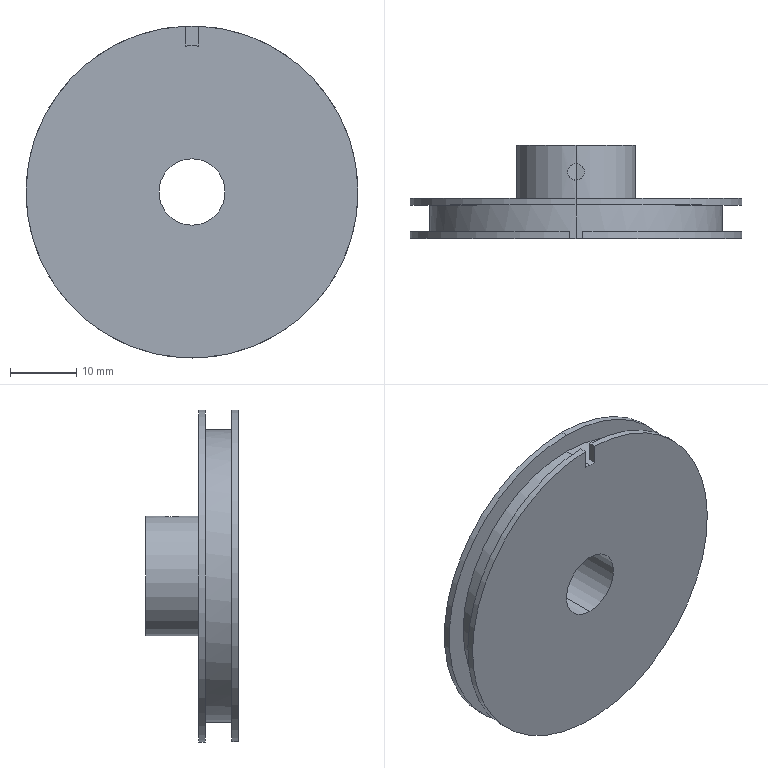Part | SolidWorks | features 3DProfileFeature 1, HoleWzd 1, ICE 1, Revolution 1 | 1 solid | 18 faces | box 50 x 14 x 50 mm | volume 10920 mm3 | cylinder 11 | plane 7 | commonest cylinder face diameters 50 x3 2.5 x2 10 x2 18 x2 44 x2
STEP:
#1=CARTESIAN_POINT('',(0.,-5.25,5.));
#2=VERTEX_POINT('',#1);
#3=CARTESIAN_POINT('',(-1.25,-4.,4.841));
#4=VERTEX_POINT('',#3);
#5=CARTESIAN_POINT('',(0.,-5.25,5.));
#6=CARTESIAN_POINT('',(-0.1659,-5.25,5.));
#7=CARTESIAN_POINT('',(-0.3287,-5.217,4.991));
#8=CARTESIAN_POINT('',(-0.6313,-5.091,4.962));
#9=CARTESIAN_POINT('',(-0.7695,-4.998,4.942));
#10=CARTESIAN_POINT('',(-0.9991,-4.769,4.901));
#11=CARTESIAN_POINT('',(-1.092,-4.63,4.88));
#12=CARTESIAN_POINT('',(-1.217,-4.329,4.85));
#13=CARTESIAN_POINT('',(-1.25,-4.164,4.841));
#14=CARTESIAN_POINT('',(-1.25,-4.,4.841));
#15=B_SPLINE_CURVE_WITH_KNOTS('',3,(#5,#6,#7,#8,#9,#10,#11,#12,#13,#14),.UNSPECIFIED.,.F.,.F.,(4,2,2,2,4),(0.,0.0004906,0.0009812,0.001472,0.001962),.UNSPECIFIED.);
#16=EDGE_CURVE('',#2,#4,#15,.T.);
#17=ORIENTED_EDGE('',*,*,#16,.T.);
#18=CARTESIAN_POINT('',(-1.25,-4.,8.913));
#19=VERTEX_POINT('',#18);
#20=CARTESIAN_POINT('',(-1.25,-4.,9.));
#21=DIRECTION('',(0.,0.,1.));
#22=VECTOR('',#21,1000.);
#23=LINE('',#20,#22);
#24=EDGE_CURVE('',#4,#19,#23,.T.);
#25=ORIENTED_EDGE('',*,*,#24,.T.);
#26=CARTESIAN_POINT('',(0.,-5.25,9.));
#27=VERTEX_POINT('',#26);
#28=CARTESIAN_POINT('',(-1.25,-4.,8.913));
#29=CARTESIAN_POINT('',(-1.25,-4.165,8.913));
#30=CARTESIAN_POINT('',(-1.217,-4.328,8.918));
#31=CARTESIAN_POINT('',(-1.092,-4.63,8.934));
#32=CARTESIAN_POINT('',(-0.9992,-4.768,8.945));
#33=CARTESIAN_POINT('',(-0.7692,-4.999,8.968));
#34=CARTESIAN_POINT('',(-0.63,-5.092,8.979));
#35=CARTESIAN_POINT('',(-0.3295,-5.217,8.995));
#36=CARTESIAN_POINT('',(-0.1653,-5.25,9.));
#37=CARTESIAN_POINT('',(0.,-5.25,9.));
#38=B_SPLINE_CURVE_WITH_KNOTS('',3,(#28,#29,#30,#31,#32,#33,#34,#35,#36,#37),.UNSPECIFIED.,.F.,.F.,(4,2,2,2,4),(0.00587,0.006358,0.006847,0.007336,0.007825),.UNSPECIFIED.);
#39=EDGE_CURVE('',#19,#27,#38,.T.);
#40=ORIENTED_EDGE('',*,*,#39,.T.);
#41=CARTESIAN_POINT('',(1.25,-4.,8.913));
#42=VERTEX_POINT('',#41);
#43=CARTESIAN_POINT('',(0.,-5.25,9.));
#44=CARTESIAN_POINT('',(0.1654,-5.25,9.));
#45=CARTESIAN_POINT('',(0.3278,-5.217,8.995));
#46=CARTESIAN_POINT('',(0.6305,-5.092,8.979));
#47=CARTESIAN_POINT('',(0.7691,-4.999,8.968));
#48=CARTESIAN_POINT('',(0.9994,-4.768,8.945));
#49=CARTESIAN_POINT('',(1.092,-4.629,8.934));
#50=CARTESIAN_POINT('',(1.217,-4.328,8.918));
#51=CARTESIAN_POINT('',(1.25,-4.163,8.913));
#52=CARTESIAN_POINT('',(1.25,-4.,8.913));
#53=B_SPLINE_CURVE_WITH_KNOTS('',3,(#43,#44,#45,#46,#47,#48,#49,#50,#51,#52),.UNSPECIFIED.,.F.,.F.,(4,2,2,2,4),(0.,0.0004892,0.0009784,0.001468,0.001957),.UNSPECIFIED.);
#54=EDGE_CURVE('',#27,#42,#53,.T.);
#55=ORIENTED_EDGE('',*,*,#54,.T.);
#56=CARTESIAN_POINT('',(1.25,-4.,4.841));
#57=VERTEX_POINT('',#56);
#58=CARTESIAN_POINT('',(1.25,-4.,9.));
#59=DIRECTION('',(0.,0.,1.));
#60=VECTOR('',#59,1000.);
#61=LINE('',#58,#60);
#62=EDGE_CURVE('',#57,#42,#61,.T.);
#63=ORIENTED_EDGE('',*,*,#62,.F.);
#64=CARTESIAN_POINT('',(1.25,-4.,4.841));
#65=CARTESIAN_POINT('',(1.25,-4.082,4.841));
#66=CARTESIAN_POINT('',(1.242,-4.164,4.843));
#67=CARTESIAN_POINT('',(1.21,-4.324,4.851));
#68=CARTESIAN_POINT('',(1.186,-4.404,4.857));
#69=CARTESIAN_POINT('',(1.092,-4.63,4.88));
#70=CARTESIAN_POINT('',(0.9989,-4.769,4.901));
#71=CARTESIAN_POINT('',(0.7696,-4.998,4.942));
#72=CARTESIAN_POINT('',(0.6309,-5.091,4.962));
#73=CARTESIAN_POINT('',(0.3301,-5.217,4.991));
#74=CARTESIAN_POINT('',(0.1658,-5.25,5.));
#75=CARTESIAN_POINT('',(0.,-5.25,5.));
#76=B_SPLINE_CURVE_WITH_KNOTS('',3,(#64,#65,#66,#67,#68,#69,#70,#71,#72,#73,#74,#75),.UNSPECIFIED.,.F.,.F.,(4,2,2,2,2,4),(0.005885,0.006131,0.006376,0.006866,0.007356,0.007846),.UNSPECIFIED.);
#77=EDGE_CURVE('',#57,#2,#76,.T.);
#78=ORIENTED_EDGE('',*,*,#77,.T.);
#79=EDGE_LOOP('',(#17,#25,#40,#55,#63,#78));
#80=FACE_OUTER_BOUND('',#79,.T.);
#81=CARTESIAN_POINT('',(0.,-4.,9.));
#82=DIRECTION('',(0.,0.,1.));
#83=DIRECTION('',(1.,0.,0.));
#84=AXIS2_PLACEMENT_3D('',#81,#82,#83);
#85=CYLINDRICAL_SURFACE('',#84,1.25);
#86=ADVANCED_FACE('',(#80),#85,.F.);
#87=CARTESIAN_POINT('',(1.,-13.,21.977));
#88=VERTEX_POINT('',#87);
#89=CARTESIAN_POINT('',(0.,-13.,-22.));
#90=VERTEX_POINT('',#89);
#91=CARTESIAN_POINT('',(0.,-13.,0.));
#92=DIRECTION('',(0.,1.,0.));
#93=DIRECTION('',(0.,0.,1.));
#94=AXIS2_PLACEMENT_3D('',#91,#92,#93);
#95=CIRCLE('',#94,22.);
#96=EDGE_CURVE('',#88,#90,#95,.T.);
#97=ORIENTED_EDGE('',*,*,#96,.T.);
#98=CARTESIAN_POINT('',(0.,-9.,-22.));
#99=VERTEX_POINT('',#98);
#100=CARTESIAN_POINT('',(0.,0.,-22.));
#101=DIRECTION('',(0.,1.,0.));
#102=VECTOR('',#101,1000.);
#103=LINE('',#100,#102);
#104=EDGE_CURVE('',#90,#99,#103,.T.);
#105=ORIENTED_EDGE('',*,*,#104,.T.);
#106=CARTESIAN_POINT('',(0.,-9.,22.));
#107=VERTEX_POINT('',#106);
#108=CARTESIAN_POINT('',(0.,-9.,0.));
#109=DIRECTION('',(0.,1.,0.));
#110=DIRECTION('',(0.,0.,1.));
#111=AXIS2_PLACEMENT_3D('',#108,#109,#110);
#112=CIRCLE('',#111,22.);
#113=EDGE_CURVE('',#107,#99,#112,.T.);
#114=ORIENTED_EDGE('',*,*,#113,.F.);
#115=CARTESIAN_POINT('',(0.,-14.,22.));
#116=VERTEX_POINT('',#115);
#117=CARTESIAN_POINT('',(0.,0.,22.));
#118=DIRECTION('',(0.,1.,0.));
#119=VECTOR('',#118,1000.);
#120=LINE('',#117,#119);
#121=EDGE_CURVE('',#116,#107,#120,.T.);
#122=ORIENTED_EDGE('',*,*,#121,.F.);
#123=CARTESIAN_POINT('',(1.,-14.,21.977));
#124=VERTEX_POINT('',#123);
#125=CARTESIAN_POINT('',(0.,-14.,0.));
#126=DIRECTION('',(0.,1.,0.));
#127=DIRECTION('',(0.,0.,-1.));
#128=AXIS2_PLACEMENT_3D('',#125,#126,#127);
#129=CIRCLE('',#128,22.);
#130=EDGE_CURVE('',#116,#124,#129,.T.);
#131=ORIENTED_EDGE('',*,*,#130,.T.);
#132=CARTESIAN_POINT('',(1.,-23.,21.977));
#133=DIRECTION('',(0.,1.,0.));
#134=VECTOR('',#133,1000.);
#135=LINE('',#132,#134);
#136=EDGE_CURVE('',#124,#88,#135,.T.);
#137=ORIENTED_EDGE('',*,*,#136,.T.);
#138=EDGE_LOOP('',(#97,#105,#114,#122,#131,#137));
#139=FACE_OUTER_BOUND('',#138,.T.);
#140=CARTESIAN_POINT('',(0.,0.,0.));
#141=DIRECTION('',(0.,1.,0.));
#142=DIRECTION('',(0.,0.,1.));
#143=AXIS2_PLACEMENT_3D('',#140,#141,#142);
#144=CYLINDRICAL_SURFACE('',#143,22.);
#145=ADVANCED_FACE('',(#139),#144,.T.);
#146=CARTESIAN_POINT('',(0.,-9.,25.));
#147=VERTEX_POINT('',#146);
#148=CARTESIAN_POINT('',(0.,-9.,-25.));
#149=VERTEX_POINT('',#148);
#150=CARTESIAN_POINT('',(0.,-9.,0.));
#151=DIRECTION('',(0.,1.,0.));
#152=DIRECTION('',(0.,0.,1.));
#153=AXIS2_PLACEMENT_3D('',#150,#151,#152);
#154=CIRCLE('',#153,25.);
#155=EDGE_CURVE('',#147,#149,#154,.T.);
#156=ORIENTED_EDGE('',*,*,#155,.T.);
#157=CARTESIAN_POINT('',(0.,-8.,-25.));
#158=VERTEX_POINT('',#157);
#159=CARTESIAN_POINT('',(0.,0.,-25.));
#160=DIRECTION('',(0.,1.,0.));
#161=VECTOR('',#160,1000.);
#162=LINE('',#159,#161);
#163=EDGE_CURVE('',#149,#158,#162,.T.);
#164=ORIENTED_EDGE('',*,*,#163,.T.);
#165=CARTESIAN_POINT('',(0.,-8.,25.));
#166=VERTEX_POINT('',#165);
#167=CARTESIAN_POINT('',(0.,-8.,0.));
#168=DIRECTION('',(0.,1.,0.));
#169=DIRECTION('',(0.,0.,1.));
#170=AXIS2_PLACEMENT_3D('',#167,#168,#169);
#171=CIRCLE('',#170,25.);
#172=EDGE_CURVE('',#166,#158,#171,.T.);
#173=ORIENTED_EDGE('',*,*,#172,.F.);
#174=CARTESIAN_POINT('',(0.,0.,25.));
#175=DIRECTION('',(0.,1.,0.));
#176=VECTOR('',#175,1000.);
#177=LINE('',#174,#176);
#178=EDGE_CURVE('',#147,#166,#177,.T.);
#179=ORIENTED_EDGE('',*,*,#178,.F.);
#180=EDGE_LOOP('',(#156,#164,#173,#179));
#181=FACE_OUTER_BOUND('',#180,.T.);
#182=CARTESIAN_POINT('',(0.,0.,0.));
#183=DIRECTION('',(0.,1.,0.));
#184=DIRECTION('',(0.,0.,1.));
#185=AXIS2_PLACEMENT_3D('',#182,#183,#184);
#186=CYLINDRICAL_SURFACE('',#185,25.);
#187=ADVANCED_FACE('',(#181),#186,.T.);
#188=CARTESIAN_POINT('',(0.,-8.,9.));
#189=VERTEX_POINT('',#188);
#190=CARTESIAN_POINT('',(0.,-8.,-9.));
#191=VERTEX_POINT('',#190);
#192=CARTESIAN_POINT('',(0.,-8.,0.));
#193=DIRECTION('',(0.,1.,0.));
#194=DIRECTION('',(0.,0.,1.));
#195=AXIS2_PLACEMENT_3D('',#192,#193,#194);
#196=CIRCLE('',#195,9.);
#197=EDGE_CURVE('',#189,#191,#196,.T.);
#198=ORIENTED_EDGE('',*,*,#197,.T.);
#199=CARTESIAN_POINT('',(0.,0.,-9.));
#200=VERTEX_POINT('',#199);
#201=CARTESIAN_POINT('',(0.,0.,-9.));
#202=DIRECTION('',(0.,1.,0.));
#203=VECTOR('',#202,1000.);
#204=LINE('',#201,#203);
#205=EDGE_CURVE('',#191,#200,#204,.T.);
#206=ORIENTED_EDGE('',*,*,#205,.T.);
#207=CARTESIAN_POINT('',(0.,0.,9.));
#208=VERTEX_POINT('',#207);
#209=CARTESIAN_POINT('',(0.,0.,0.));
#210=DIRECTION('',(0.,1.,0.));
#211=DIRECTION('',(0.,0.,1.));
#212=AXIS2_PLACEMENT_3D('',#209,#210,#211);
#213=CIRCLE('',#212,9.);
#214=EDGE_CURVE('',#208,#200,#213,.T.);
#215=ORIENTED_EDGE('',*,*,#214,.F.);
#216=CARTESIAN_POINT('',(0.,-2.75,9.));
#217=VERTEX_POINT('',#216);
#218=CARTESIAN_POINT('',(0.,0.,9.));
#219=DIRECTION('',(0.,1.,0.));
#220=VECTOR('',#219,1000.);
#221=LINE('',#218,#220);
#222=EDGE_CURVE('',#217,#208,#221,.T.);
#223=ORIENTED_EDGE('',*,*,#222,.F.);
#224=CARTESIAN_POINT('',(1.25,-4.,8.913));
#225=CARTESIAN_POINT('',(1.25,-3.918,8.913));
#226=CARTESIAN_POINT('',(1.242,-3.835,8.914));
#227=CARTESIAN_POINT('',(1.21,-3.675,8.918));
#228=CARTESIAN_POINT('',(1.186,-3.597,8.922));
#229=CARTESIAN_POINT('',(1.092,-3.37,8.934));
#230=CARTESIAN_POINT('',(1.,-3.233,8.945));
#231=CARTESIAN_POINT('',(0.7672,-3.,8.968));
#232=CARTESIAN_POINT('',(0.6297,-2.908,8.979));
#233=CARTESIAN_POINT('',(0.4028,-2.814,8.991));
#234=CARTESIAN_POINT('',(0.3249,-2.79,8.994));
#235=CARTESIAN_POINT('',(0.1645,-2.758,8.999));
#236=CARTESIAN_POINT('',(0.08161,-2.75,9.));
#237=CARTESIAN_POINT('',(0.,-2.75,9.));
#238=B_SPLINE_CURVE_WITH_KNOTS('',3,(#224,#225,#226,#227,#228,#229,#230,#231,#232,#233,#234,#235,#236,#237),.UNSPECIFIED.,.F.,.F.,(4,2,2,2,2,2,4),(0.001957,0.002201,0.002446,0.002935,0.003424,0.003668,0.003913),.UNSPECIFIED.);
#239=EDGE_CURVE('',#42,#217,#238,.T.);
#240=ORIENTED_EDGE('',*,*,#239,.F.);
#241=ORIENTED_EDGE('',*,*,#54,.F.);
#242=CARTESIAN_POINT('',(0.,0.,9.));
#243=DIRECTION('',(0.,1.,0.));
#244=VECTOR('',#243,1000.);
#245=LINE('',#242,#244);
#246=EDGE_CURVE('',#189,#27,#245,.T.);
#247=ORIENTED_EDGE('',*,*,#246,.F.);
#248=EDGE_LOOP('',(#198,#206,#215,#223,#240,#241,#247));
#249=FACE_OUTER_BOUND('',#248,.T.);
#250=CARTESIAN_POINT('',(0.,0.,0.));
#251=DIRECTION('',(0.,1.,0.));
#252=DIRECTION('',(0.,0.,1.));
#253=AXIS2_PLACEMENT_3D('',#250,#251,#252);
#254=CYLINDRICAL_SURFACE('',#253,9.);
#255=ADVANCED_FACE('',(#249),#254,.T.);
#256=CARTESIAN_POINT('',(0.,-14.,-5.));
#257=VERTEX_POINT('',#256);
#258=CARTESIAN_POINT('',(0.,-14.,5.));
#259=VERTEX_POINT('',#258);
#260=CARTESIAN_POINT('',(0.,-14.,0.));
#261=DIRECTION('',(0.,1.,0.));
#262=DIRECTION('',(0.,0.,1.));
#263=AXIS2_PLACEMENT_3D('',#260,#261,#262);
#264=CIRCLE('',#263,5.);
#265=EDGE_CURVE('',#257,#259,#264,.T.);
#266=ORIENTED_EDGE('',*,*,#265,.F.);
#267=CARTESIAN_POINT('',(0.,0.,-5.));
#268=VERTEX_POINT('',#267);
#269=CARTESIAN_POINT('',(0.,0.,-5.));
#270=DIRECTION('',(0.,1.,0.));
#271=VECTOR('',#270,1000.);
#272=LINE('',#269,#271);
#273=EDGE_CURVE('',#257,#268,#272,.T.);
#274=ORIENTED_EDGE('',*,*,#273,.T.);
#275=CARTESIAN_POINT('',(0.,0.,5.));
#276=VERTEX_POINT('',#275);
#277=CARTESIAN_POINT('',(0.,0.,0.));
#278=DIRECTION('',(0.,1.,0.));
#279=DIRECTION('',(0.,0.,1.));
#280=AXIS2_PLACEMENT_3D('',#277,#278,#279);
#281=CIRCLE('',#280,5.);
#282=EDGE_CURVE('',#268,#276,#281,.T.);
#283=ORIENTED_EDGE('',*,*,#282,.T.);
#284=CARTESIAN_POINT('',(0.,-2.75,5.));
#285=VERTEX_POINT('',#284);
#286=CARTESIAN_POINT('',(0.,0.,5.));
#287=DIRECTION('',(0.,1.,0.));
#288=VECTOR('',#287,1000.);
#289=LINE('',#286,#288);
#290=EDGE_CURVE('',#285,#276,#289,.T.);
#291=ORIENTED_EDGE('',*,*,#290,.F.);
#292=CARTESIAN_POINT('',(-1.25,-4.,4.841));
#293=CARTESIAN_POINT('',(-1.25,-3.918,4.841));
#294=CARTESIAN_POINT('',(-1.242,-3.835,4.843));
#295=CARTESIAN_POINT('',(-1.21,-3.674,4.852));
#296=CARTESIAN_POINT('',(-1.186,-3.596,4.857));
#297=CARTESIAN_POINT('',(-1.091,-3.369,4.88));
#298=CARTESIAN_POINT('',(-0.9993,-3.231,4.901));
#299=CARTESIAN_POINT('',(-0.8256,-3.058,4.932));
#300=CARTESIAN_POINT('',(-0.7628,-3.006,4.942));
#301=CARTESIAN_POINT('',(-0.6277,-2.916,4.961));
#302=CARTESIAN_POINT('',(-0.5545,-2.877,4.97));
#303=CARTESIAN_POINT('',(-0.3282,-2.783,4.992));
#304=CARTESIAN_POINT('',(-0.1635,-2.75,5.));
#305=CARTESIAN_POINT('',(0.,-2.75,5.));
#306=B_SPLINE_CURVE_WITH_KNOTS('',3,(#292,#293,#294,#295,#296,#297,#298,#299,#300,#301,#302,#303,#304,#305),.UNSPECIFIED.,.F.,.F.,(4,2,2,2,2,2,4),(0.001962,0.002208,0.002453,0.002943,0.003188,0.003433,0.003924),.UNSPECIFIED.);
#307=EDGE_CURVE('',#4,#285,#306,.T.);
#308=ORIENTED_EDGE('',*,*,#307,.F.);
#309=ORIENTED_EDGE('',*,*,#16,.F.);
#310=CARTESIAN_POINT('',(0.,0.,5.));
#311=DIRECTION('',(0.,1.,0.));
#312=VECTOR('',#311,1000.);
#313=LINE('',#310,#312);
#314=EDGE_CURVE('',#259,#2,#313,.T.);
#315=ORIENTED_EDGE('',*,*,#314,.F.);
#316=EDGE_LOOP('',(#266,#274,#283,#291,#308,#309,#315));
#317=FACE_OUTER_BOUND('',#316,.T.);
#318=CARTESIAN_POINT('',(0.,0.,0.));
#319=DIRECTION('',(0.,1.,0.));
#320=DIRECTION('',(0.,0.,1.));
#321=AXIS2_PLACEMENT_3D('',#318,#319,#320);
#322=CYLINDRICAL_SURFACE('',#321,5.);
#323=ADVANCED_FACE('',(#317),#322,.F.);
#324=CARTESIAN_POINT('',(0.,-14.,0.));
#325=DIRECTION('',(0.,1.,0.));
#326=DIRECTION('',(0.,0.,1.));
#327=AXIS2_PLACEMENT_3D('',#324,#325,#326);
#328=CIRCLE('',#327,5.);
#329=EDGE_CURVE('',#259,#257,#328,.T.);
#330=ORIENTED_EDGE('',*,*,#329,.T.);
#331=ORIENTED_EDGE('',*,*,#265,.T.);
#332=EDGE_LOOP('',(#330,#331));
#333=FACE_BOUND('',#332,.T.);
#334=CARTESIAN_POINT('',(1.,-14.,24.98));
#335=VERTEX_POINT('',#334);
#336=CARTESIAN_POINT('',(1.,-14.,0.));
#337=DIRECTION('',(0.,0.,1.));
#338=VECTOR('',#337,1000.);
#339=LINE('',#336,#338);
#340=EDGE_CURVE('',#124,#335,#339,.T.);
#341=ORIENTED_EDGE('',*,*,#340,.F.);
#342=ORIENTED_EDGE('',*,*,#130,.F.);
#343=CARTESIAN_POINT('',(-1.,-14.,21.977));
#344=VERTEX_POINT('',#343);
#345=CARTESIAN_POINT('',(0.,-14.,0.));
#346=DIRECTION('',(0.,1.,0.));
#347=DIRECTION('',(0.,0.,-1.));
#348=AXIS2_PLACEMENT_3D('',#345,#346,#347);
#349=CIRCLE('',#348,22.);
#350=EDGE_CURVE('',#344,#116,#349,.T.);
#351=ORIENTED_EDGE('',*,*,#350,.F.);
#352=CARTESIAN_POINT('',(-1.,-14.,24.98));
#353=VERTEX_POINT('',#352);
#354=CARTESIAN_POINT('',(-1.,-14.,0.));
#355=DIRECTION('',(0.,0.,-1.));
#356=VECTOR('',#355,1000.);
#357=LINE('',#354,#356);
#358=EDGE_CURVE('',#353,#344,#357,.T.);
#359=ORIENTED_EDGE('',*,*,#358,.F.);
#360=CARTESIAN_POINT('',(0.,-14.,0.));
#361=DIRECTION('',(0.,1.,0.));
#362=DIRECTION('',(0.,0.,1.));
#363=AXIS2_PLACEMENT_3D('',#360,#361,#362);
#364=CIRCLE('',#363,25.);
#365=EDGE_CURVE('',#335,#353,#364,.T.);
#366=ORIENTED_EDGE('',*,*,#365,.F.);
#367=EDGE_LOOP('',(#341,#342,#351,#359,#366));
#368=FACE_OUTER_BOUND('',#367,.T.);
#369=CARTESIAN_POINT('',(-25.,-14.,0.));
#370=DIRECTION('',(0.,-1.,0.));
#371=DIRECTION('',(0.,0.,-1.));
#372=AXIS2_PLACEMENT_3D('',#369,#370,#371);
#373=PLANE('',#372);
#374=ADVANCED_FACE('',(#333,#368),#373,.T.);
#375=ORIENTED_EDGE('',*,*,#273,.F.);
#376=ORIENTED_EDGE('',*,*,#329,.F.);
#377=ORIENTED_EDGE('',*,*,#314,.T.);
#378=ORIENTED_EDGE('',*,*,#77,.F.);
#379=CARTESIAN_POINT('',(0.,-2.75,5.));
#380=CARTESIAN_POINT('',(0.1635,-2.75,5.));
#381=CARTESIAN_POINT('',(0.3287,-2.783,4.991));
#382=CARTESIAN_POINT('',(0.6298,-2.908,4.962));
#383=CARTESIAN_POINT('',(0.7684,-3.001,4.942));
#384=CARTESIAN_POINT('',(0.999,-3.231,4.901));
#385=CARTESIAN_POINT('',(1.091,-3.368,4.88));
#386=CARTESIAN_POINT('',(1.217,-3.672,4.85));
#387=CARTESIAN_POINT('',(1.25,-3.835,4.841));
#388=CARTESIAN_POINT('',(1.25,-4.,4.841));
#389=B_SPLINE_CURVE_WITH_KNOTS('',3,(#379,#380,#381,#382,#383,#384,#385,#386,#387,#388),.UNSPECIFIED.,.F.,.F.,(4,2,2,2,4),(0.003924,0.004414,0.004905,0.005395,0.005885),.UNSPECIFIED.);
#390=EDGE_CURVE('',#285,#57,#389,.T.);
#391=ORIENTED_EDGE('',*,*,#390,.F.);
#392=ORIENTED_EDGE('',*,*,#290,.T.);
#393=CARTESIAN_POINT('',(0.,0.,0.));
#394=DIRECTION('',(0.,1.,0.));
#395=DIRECTION('',(0.,0.,1.));
#396=AXIS2_PLACEMENT_3D('',#393,#394,#395);
#397=CIRCLE('',#396,5.);
#398=EDGE_CURVE('',#276,#268,#397,.T.);
#399=ORIENTED_EDGE('',*,*,#398,.T.);
#400=EDGE_LOOP('',(#375,#376,#377,#378,#391,#392,#399));
#401=FACE_OUTER_BOUND('',#400,.T.);
#402=CARTESIAN_POINT('',(0.,0.,0.));
#403=DIRECTION('',(0.,1.,0.));
#404=DIRECTION('',(0.,0.,1.));
#405=AXIS2_PLACEMENT_3D('',#402,#403,#404);
#406=CYLINDRICAL_SURFACE('',#405,5.);
#407=ADVANCED_FACE('',(#401),#406,.F.);
#408=ORIENTED_EDGE('',*,*,#214,.T.);
#409=CARTESIAN_POINT('',(0.,0.,0.));
#410=DIRECTION('',(0.,1.,0.));
#411=DIRECTION('',(0.,0.,1.));
#412=AXIS2_PLACEMENT_3D('',#409,#410,#411);
#413=CIRCLE('',#412,9.);
#414=EDGE_CURVE('',#200,#208,#413,.T.);
#415=ORIENTED_EDGE('',*,*,#414,.T.);
#416=EDGE_LOOP('',(#408,#415));
#417=FACE_OUTER_BOUND('',#416,.T.);
#418=ORIENTED_EDGE('',*,*,#398,.F.);
#419=ORIENTED_EDGE('',*,*,#282,.F.);
#420=EDGE_LOOP('',(#418,#419));
#421=FACE_BOUND('',#420,.T.);
#422=CARTESIAN_POINT('',(-5.,0.,0.));
#423=DIRECTION('',(0.,1.,0.));
#424=DIRECTION('',(0.,0.,1.));
#425=AXIS2_PLACEMENT_3D('',#422,#423,#424);
#426=PLANE('',#425);
#427=ADVANCED_FACE('',(#417,#421),#426,.T.);
#428=ORIENTED_EDGE('',*,*,#205,.F.);
#429=CARTESIAN_POINT('',(0.,-8.,0.));
#430=DIRECTION('',(0.,1.,0.));
#431=DIRECTION('',(0.,0.,1.));
#432=AXIS2_PLACEMENT_3D('',#429,#430,#431);
#433=CIRCLE('',#432,9.);
#434=EDGE_CURVE('',#191,#189,#433,.T.);
#435=ORIENTED_EDGE('',*,*,#434,.T.);
#436=ORIENTED_EDGE('',*,*,#246,.T.);
#437=ORIENTED_EDGE('',*,*,#39,.F.);
#438=CARTESIAN_POINT('',(0.,-2.75,9.));
#439=CARTESIAN_POINT('',(-0.1633,-2.75,9.));
#440=CARTESIAN_POINT('',(-0.328,-2.783,8.995));
#441=CARTESIAN_POINT('',(-0.629,-2.908,8.979));
#442=CARTESIAN_POINT('',(-0.7683,-3.001,8.968));
#443=CARTESIAN_POINT('',(-0.9413,-3.173,8.951));
#444=CARTESIAN_POINT('',(-0.994,-3.238,8.945));
#445=CARTESIAN_POINT('',(-1.085,-3.373,8.935));
#446=CARTESIAN_POINT('',(-1.123,-3.445,8.93));
#447=CARTESIAN_POINT('',(-1.217,-3.672,8.918));
#448=CARTESIAN_POINT('',(-1.25,-3.835,8.913));
#449=CARTESIAN_POINT('',(-1.25,-4.,8.913));
#450=B_SPLINE_CURVE_WITH_KNOTS('',3,(#438,#439,#440,#441,#442,#443,#444,#445,#446,#447,#448,#449),.UNSPECIFIED.,.F.,.F.,(4,2,2,2,2,4),(0.003913,0.004402,0.004891,0.005136,0.00538,0.00587),.UNSPECIFIED.);
#451=EDGE_CURVE('',#217,#19,#450,.T.);
#452=ORIENTED_EDGE('',*,*,#451,.F.);
#453=ORIENTED_EDGE('',*,*,#222,.T.);
#454=ORIENTED_EDGE('',*,*,#414,.F.);
#455=EDGE_LOOP('',(#428,#435,#436,#437,#452,#453,#454));
#456=FACE_OUTER_BOUND('',#455,.T.);
#457=CARTESIAN_POINT('',(0.,0.,0.));
#458=DIRECTION('',(0.,1.,0.));
#459=DIRECTION('',(0.,0.,1.));
#460=AXIS2_PLACEMENT_3D('',#457,#458,#459);
#461=CYLINDRICAL_SURFACE('',#460,9.);
#462=ADVANCED_FACE('',(#456),#461,.T.);
#463=ORIENTED_EDGE('',*,*,#172,.T.);
#464=CARTESIAN_POINT('',(0.,-8.,0.));
#465=DIRECTION('',(0.,1.,0.));
#466=DIRECTION('',(0.,0.,1.));
#467=AXIS2_PLACEMENT_3D('',#464,#465,#466);
#468=CIRCLE('',#467,25.);
#469=EDGE_CURVE('',#158,#166,#468,.T.);
#470=ORIENTED_EDGE('',*,*,#469,.T.);
#471=EDGE_LOOP('',(#463,#470));
#472=FACE_OUTER_BOUND('',#471,.T.);
#473=ORIENTED_EDGE('',*,*,#197,.F.);
#474=ORIENTED_EDGE('',*,*,#434,.F.);
#475=EDGE_LOOP('',(#473,#474));
#476=FACE_BOUND('',#475,.T.);
#477=CARTESIAN_POINT('',(-9.,-8.,0.));
#478=DIRECTION('',(0.,1.,0.));
#479=DIRECTION('',(0.,0.,1.));
#480=AXIS2_PLACEMENT_3D('',#477,#478,#479);
#481=PLANE('',#480);
#482=ADVANCED_FACE('',(#472,#476),#481,.T.);
#483=ORIENTED_EDGE('',*,*,#163,.F.);
#484=CARTESIAN_POINT('',(0.,-9.,0.));
#485=DIRECTION('',(0.,1.,0.));
#486=DIRECTION('',(0.,0.,1.));
#487=AXIS2_PLACEMENT_3D('',#484,#485,#486);
#488=CIRCLE('',#487,25.);
#489=EDGE_CURVE('',#149,#147,#488,.T.);
#490=ORIENTED_EDGE('',*,*,#489,.T.);
#491=ORIENTED_EDGE('',*,*,#178,.T.);
#492=ORIENTED_EDGE('',*,*,#469,.F.);
#493=EDGE_LOOP('',(#483,#490,#491,#492));
#494=FACE_OUTER_BOUND('',#493,.T.);
#495=CARTESIAN_POINT('',(0.,0.,0.));
#496=DIRECTION('',(0.,1.,0.));
#497=DIRECTION('',(0.,0.,1.));
#498=AXIS2_PLACEMENT_3D('',#495,#496,#497);
#499=CYLINDRICAL_SURFACE('',#498,25.);
#500=ADVANCED_FACE('',(#494),#499,.T.);
#501=ORIENTED_EDGE('',*,*,#113,.T.);
#502=CARTESIAN_POINT('',(0.,-9.,0.));
#503=DIRECTION('',(0.,1.,0.));
#504=DIRECTION('',(0.,0.,1.));
#505=AXIS2_PLACEMENT_3D('',#502,#503,#504);
#506=CIRCLE('',#505,22.);
#507=EDGE_CURVE('',#99,#107,#506,.T.);
#508=ORIENTED_EDGE('',*,*,#507,.T.);
#509=EDGE_LOOP('',(#501,#508));
#510=FACE_BOUND('',#509,.T.);
#511=ORIENTED_EDGE('',*,*,#155,.F.);
#512=ORIENTED_EDGE('',*,*,#489,.F.);
#513=EDGE_LOOP('',(#511,#512));
#514=FACE_OUTER_BOUND('',#513,.T.);
#515=CARTESIAN_POINT('',(-25.,-9.,0.));
#516=DIRECTION('',(0.,-1.,0.));
#517=DIRECTION('',(0.,0.,-1.));
#518=AXIS2_PLACEMENT_3D('',#515,#516,#517);
#519=PLANE('',#518);
#520=ADVANCED_FACE('',(#510,#514),#519,.T.);
#521=ORIENTED_EDGE('',*,*,#104,.F.);
#522=CARTESIAN_POINT('',(-1.,-13.,21.977));
#523=VERTEX_POINT('',#522);
#524=CARTESIAN_POINT('',(0.,-13.,0.));
#525=DIRECTION('',(0.,1.,0.));
#526=DIRECTION('',(0.,0.,1.));
#527=AXIS2_PLACEMENT_3D('',#524,#525,#526);
#528=CIRCLE('',#527,22.);
#529=EDGE_CURVE('',#90,#523,#528,.T.);
#530=ORIENTED_EDGE('',*,*,#529,.T.);
#531=CARTESIAN_POINT('',(-1.,-23.,21.977));
#532=DIRECTION('',(0.,1.,0.));
#533=VECTOR('',#532,1000.);
#534=LINE('',#531,#533);
#535=EDGE_CURVE('',#344,#523,#534,.T.);
#536=ORIENTED_EDGE('',*,*,#535,.F.);
#537=ORIENTED_EDGE('',*,*,#350,.T.);
#538=ORIENTED_EDGE('',*,*,#121,.T.);
#539=ORIENTED_EDGE('',*,*,#507,.F.);
#540=EDGE_LOOP('',(#521,#530,#536,#537,#538,#539));
#541=FACE_OUTER_BOUND('',#540,.T.);
#542=CARTESIAN_POINT('',(0.,0.,0.));
#543=DIRECTION('',(0.,1.,0.));
#544=DIRECTION('',(0.,0.,1.));
#545=AXIS2_PLACEMENT_3D('',#542,#543,#544);
#546=CYLINDRICAL_SURFACE('',#545,22.);
#547=ADVANCED_FACE('',(#541),#546,.T.);
#548=CARTESIAN_POINT('',(1.,-13.,24.98));
#549=VERTEX_POINT('',#548);
#550=CARTESIAN_POINT('',(1.,-13.,21.977));
#551=DIRECTION('',(0.,0.,-1.));
#552=VECTOR('',#551,1000.);
#553=LINE('',#550,#552);
#554=EDGE_CURVE('',#549,#88,#553,.T.);
#555=ORIENTED_EDGE('',*,*,#554,.F.);
#556=CARTESIAN_POINT('',(-1.,-13.,24.98));
#557=VERTEX_POINT('',#556);
#558=CARTESIAN_POINT('',(0.,-13.,0.));
#559=DIRECTION('',(0.,1.,0.));
#560=DIRECTION('',(0.,0.,1.));
#561=AXIS2_PLACEMENT_3D('',#558,#559,#560);
#562=CIRCLE('',#561,25.);
#563=EDGE_CURVE('',#549,#557,#562,.T.);
#564=ORIENTED_EDGE('',*,*,#563,.T.);
#565=CARTESIAN_POINT('',(-1.,-13.,21.977));
#566=DIRECTION('',(0.,0.,1.));
#567=VECTOR('',#566,1000.);
#568=LINE('',#565,#567);
#569=EDGE_CURVE('',#523,#557,#568,.T.);
#570=ORIENTED_EDGE('',*,*,#569,.F.);
#571=ORIENTED_EDGE('',*,*,#529,.F.);
#572=ORIENTED_EDGE('',*,*,#96,.F.);
#573=EDGE_LOOP('',(#555,#564,#570,#571,#572));
#574=FACE_OUTER_BOUND('',#573,.T.);
#575=CARTESIAN_POINT('',(-22.,-13.,0.));
#576=DIRECTION('',(0.,1.,0.));
#577=DIRECTION('',(0.,0.,1.));
#578=AXIS2_PLACEMENT_3D('',#575,#576,#577);
#579=PLANE('',#578);
#580=ADVANCED_FACE('',(#574),#579,.T.);
#581=CARTESIAN_POINT('',(1.,0.,24.98));
#582=DIRECTION('',(0.,1.,0.));
#583=VECTOR('',#582,1000.);
#584=LINE('',#581,#583);
#585=EDGE_CURVE('',#335,#549,#584,.T.);
#586=ORIENTED_EDGE('',*,*,#585,.F.);
#587=ORIENTED_EDGE('',*,*,#365,.T.);
#588=CARTESIAN_POINT('',(-1.,0.,24.98));
#589=DIRECTION('',(0.,-1.,0.));
#590=VECTOR('',#589,1000.);
#591=LINE('',#588,#590);
#592=EDGE_CURVE('',#557,#353,#591,.T.);
#593=ORIENTED_EDGE('',*,*,#592,.F.);
#594=ORIENTED_EDGE('',*,*,#563,.F.);
#595=EDGE_LOOP('',(#586,#587,#593,#594));
#596=FACE_OUTER_BOUND('',#595,.T.);
#597=CARTESIAN_POINT('',(0.,0.,0.));
#598=DIRECTION('',(0.,1.,0.));
#599=DIRECTION('',(0.,0.,1.));
#600=AXIS2_PLACEMENT_3D('',#597,#598,#599);
#601=CYLINDRICAL_SURFACE('',#600,25.);
#602=ADVANCED_FACE('',(#596),#601,.T.);
#603=ORIENTED_EDGE('',*,*,#585,.T.);
#604=ORIENTED_EDGE('',*,*,#554,.T.);
#605=ORIENTED_EDGE('',*,*,#136,.F.);
#606=ORIENTED_EDGE('',*,*,#340,.T.);
#607=EDGE_LOOP('',(#603,#604,#605,#606));
#608=FACE_OUTER_BOUND('',#607,.T.);
#609=CARTESIAN_POINT('',(1.,-23.,21.977));
#610=DIRECTION('',(1.,0.,0.));
#611=DIRECTION('',(0.,0.,-1.));
#612=AXIS2_PLACEMENT_3D('',#609,#610,#611);
#613=PLANE('',#612);
#614=ADVANCED_FACE('',(#608),#613,.F.);
#615=ORIENTED_EDGE('',*,*,#592,.T.);
#616=ORIENTED_EDGE('',*,*,#358,.T.);
#617=ORIENTED_EDGE('',*,*,#535,.T.);
#618=ORIENTED_EDGE('',*,*,#569,.T.);
#619=EDGE_LOOP('',(#615,#616,#617,#618));
#620=FACE_OUTER_BOUND('',#619,.T.);
#621=CARTESIAN_POINT('',(-1.,-23.,21.977));
#622=DIRECTION('',(-1.,0.,0.));
#623=DIRECTION('',(0.,0.,1.));
#624=AXIS2_PLACEMENT_3D('',#621,#622,#623);
#625=PLANE('',#624);
#626=ADVANCED_FACE('',(#620),#625,.F.);
#627=ORIENTED_EDGE('',*,*,#24,.F.);
#628=ORIENTED_EDGE('',*,*,#307,.T.);
#629=ORIENTED_EDGE('',*,*,#390,.T.);
#630=ORIENTED_EDGE('',*,*,#62,.T.);
#631=ORIENTED_EDGE('',*,*,#239,.T.);
#632=ORIENTED_EDGE('',*,*,#451,.T.);
#633=EDGE_LOOP('',(#627,#628,#629,#630,#631,#632));
#634=FACE_OUTER_BOUND('',#633,.T.);
#635=CARTESIAN_POINT('',(0.,-4.,9.));
#636=DIRECTION('',(0.,0.,1.));
#637=DIRECTION('',(1.,0.,0.));
#638=AXIS2_PLACEMENT_3D('',#635,#636,#637);
#639=CYLINDRICAL_SURFACE('',#638,1.25);
#640=ADVANCED_FACE('',(#634),#639,.F.);
#641=CLOSED_SHELL('',(#86,#145,#187,#255,#323,#374,#407,#427,#462,#482,#500,#520,#547,#580,#602,#614,#626,#640));
#642=MANIFOLD_SOLID_BREP('',#641);
#643=CARTESIAN_POINT('',(0.,0.,0.));
#644=DIRECTION('',(0.,0.,1.));
#645=DIRECTION('',(1.,0.,0.));
#646=AXIS2_PLACEMENT_3D('',#643,#644,#645);
#647=(LENGTH_UNIT()NAMED_UNIT(*)SI_UNIT(.MILLI.,.METRE.));
#648=UNCERTAINTY_MEASURE_WITH_UNIT(LENGTH_MEASURE(0.00001),#647,'','');
#649=(NAMED_UNIT(*)PLANE_ANGLE_UNIT()SI_UNIT($,.RADIAN.));
#650=(NAMED_UNIT(*)SI_UNIT($,.STERADIAN.)SOLID_ANGLE_UNIT());
#651=(GEOMETRIC_REPRESENTATION_CONTEXT(3)GLOBAL_UNCERTAINTY_ASSIGNED_CONTEXT((#648))GLOBAL_UNIT_ASSIGNED_CONTEXT((#647,#649,#650))REPRESENTATION_CONTEXT('',''));
#652=ADVANCED_BREP_SHAPE_REPRESENTATION('',(#642,#646),#651);